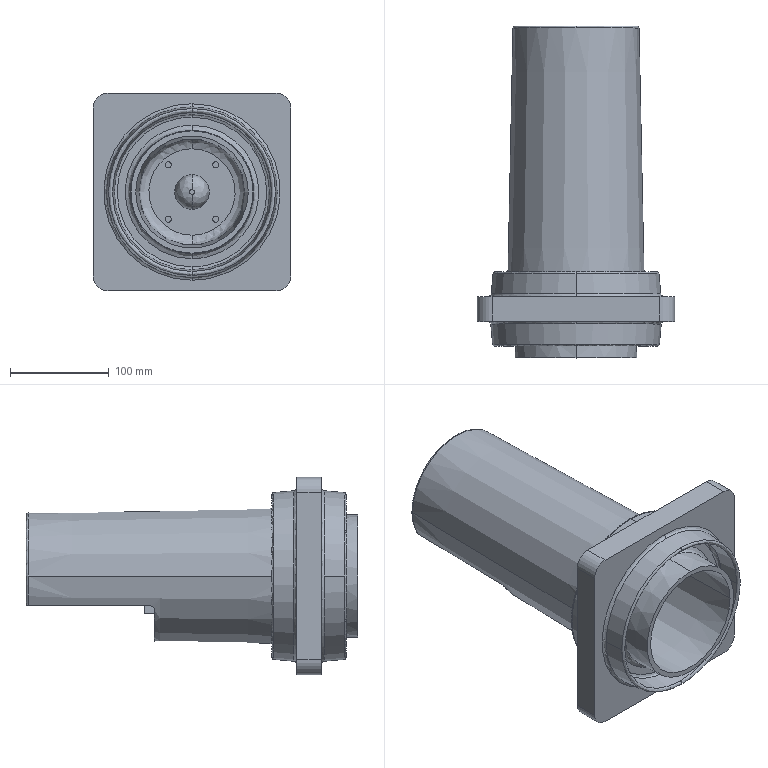Part | SolidWorks | features BaseBody 1 | 1 solid | 122 faces | box 200 x 336 x 200 mm | volume 2348409 mm3 | cylinder 42 | plane 38 | spline 26 | cone 16 | commonest cylinder face diameters 6 x8 6.3 x8 8 x8 12 x6 30 x4 10 x2